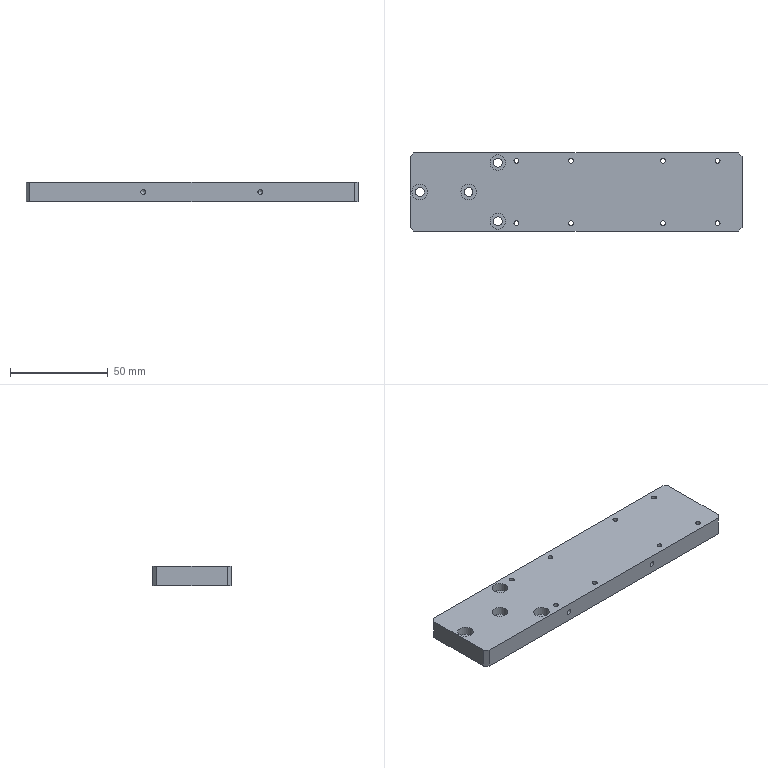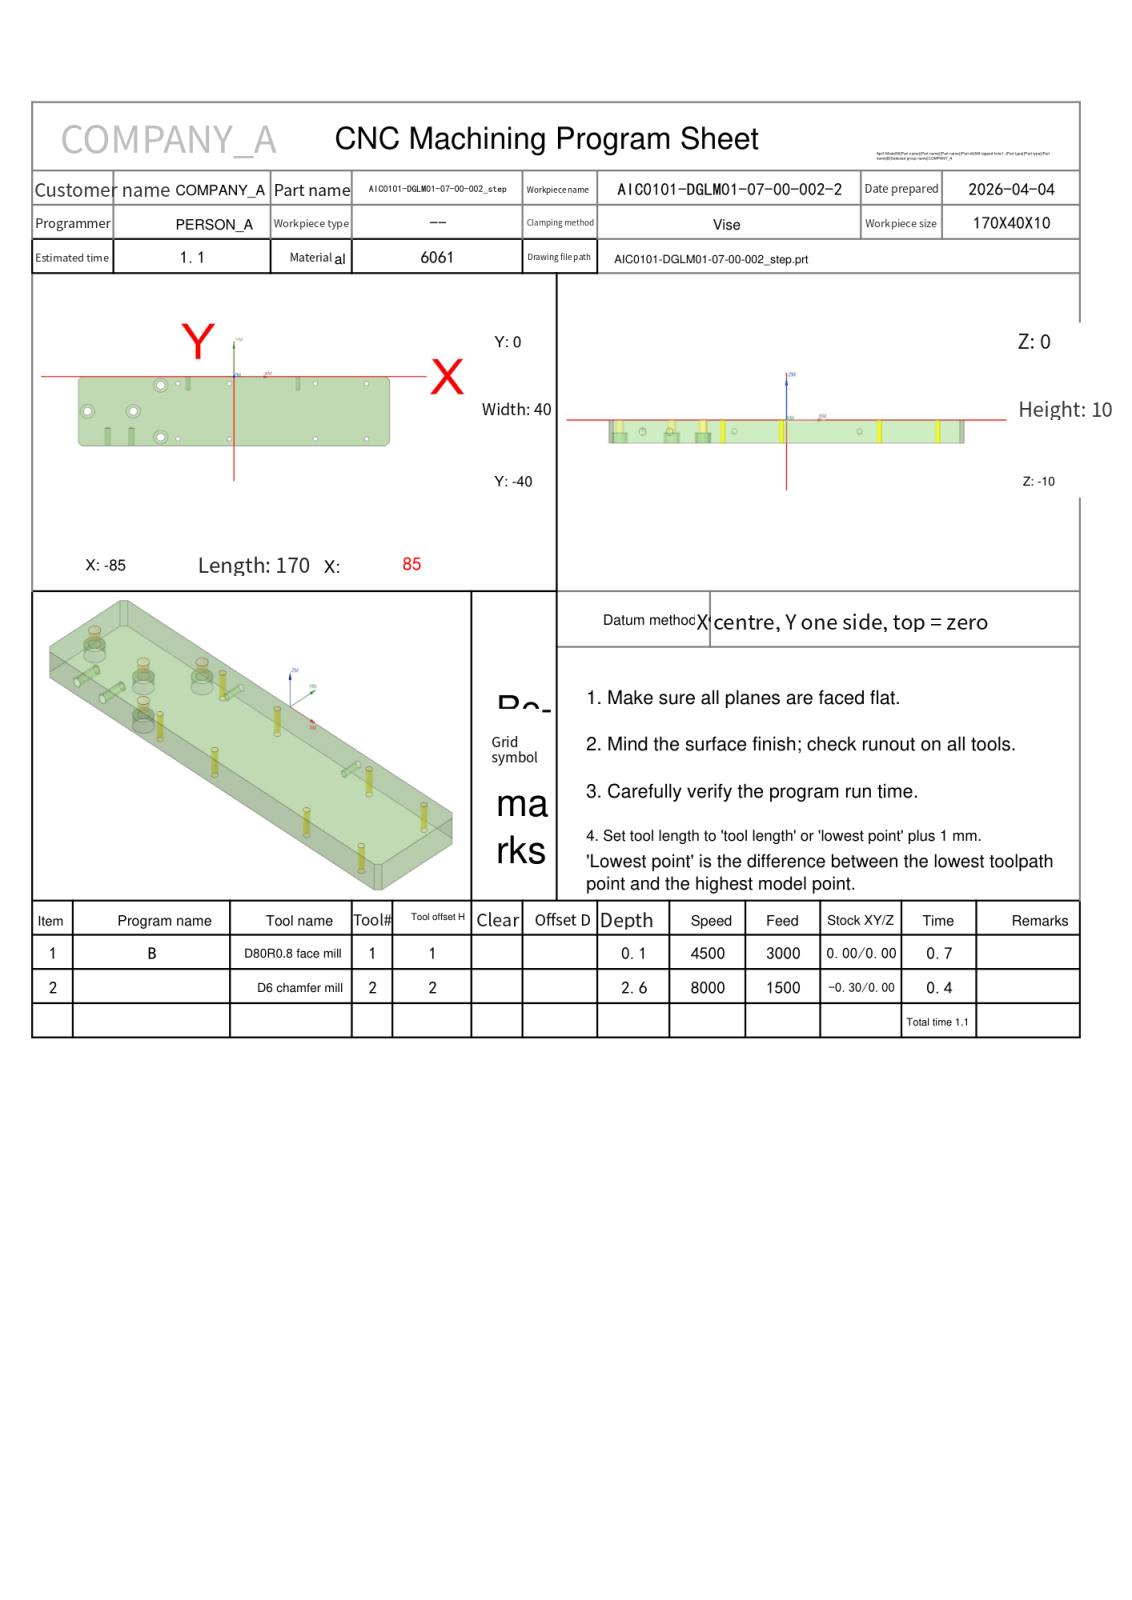NC program | NX | posted by the shop | part box 170 x 40 x 10 mm
Whole program:
%
O0001
(Machine time: 1.53 MIN)
(===Total Tool:2===)
(T1=D80R0.8 face mill D=80.  R=0.8  D-  H01 Z=0.    )
(T2=D6 chamfer mill   D=6.   R=0.   D-  H02 Z=-2.55 )
G80 G90 G17 G49 G40
G91 G28 Z0
M01
N1 T01 M06
(D80R0.8 face mill  D=80. R=0.8 H=01 ce=0.20 di=0.10)
G00 G90 G54 X137. Y-20. M03 S4500
G43 H01 Z20.
M08
Z3.525
G01 Z1.525 F3000.
X125.
X-125.
X-137.
Z3.525
G00 Z5.
X137.
Z3.05
G01 Z1.05
X125.
X-125.
X-137.
Z3.05
G00 Z4.525
X137.
Z2.575
G01 Z.575
X125.
X-125.
X-137.
Z2.575
G00 Z4.05
X137.
Z2.1
G01 Z.1
X125.
X-125.
X-137.
Z2.1
G00 Z20.
G00 G90 X137. Y-20. M03 S4500
Z20.
Z2.
G01 Z0.0 F1000.
X125.
X-125.
X-137.
Z2.
G00 Z20.
G91 G28 Z0.0
M05
M09
G91 G28 Z0.0
M01
N2 T02 M06
(D6 chamfer mill D=6. R=0. H=02 ce=0.00 di=0.00)
G00 G90 G54 X-2.5 Y-36. M03 S8000
G43 H02 Z20.
M08
G98 G81 X-2.5 Y-36. Z-1.75 R3. F1000.
X-30.5
Y-4.
X-2.5
X44.5
X72.5
Y-36.
X44.5
G80
G00 Z20.
G00 G90 X-40. Y-5. M03 S8000
Z20.
G98 G81 X-40. Y-5. Z-2.55 R3. F1000.
Y-35.
X-55. Y-20.
X-80.
G80
G00 Z20.
G00 G90 X-85.7 Y-10.954 M03 S7000
Z20.
Z2.5
G01 Y-2.047 Z-.742 F1500.
X-85.662 Y-1.84 Z-.819
X-85.581 Y-1.645 Z-.895
X-85.462 Y-1.472 Z-.972
X-85.407 Y-1.417 Z-1.
X-83.583 Y.407
G02 X-82.876 Y.7 I.707 J-.707
G01 X82.876
G02 X83.583 Y.407 I0.0 J-1.
G01 X85.407 Y-1.417
G02 X85.7 Y-2.124 I-.707 J-.707
G01 Y-37.876
G02 X85.407 Y-38.583 I-1. J0.0
G01 X83.583 Y-40.407
G02 X82.876 Y-40.7 I-.707 J.707
G01 X-82.876
G02 X-83.583 Y-40.407 I0.0 J1.
G01 X-85.407 Y-38.583
G02 X-85.7 Y-37.876 I.707 J.707
G01 Y-2.124
G02 X-85.407 Y-1.417 I1. J0.0
G01 X-85.054 Y-1.064
Z1.5
G00 Z20.
M05
M09
G91 G28 Z0.0
G91 G28 Y0.0
M30
%